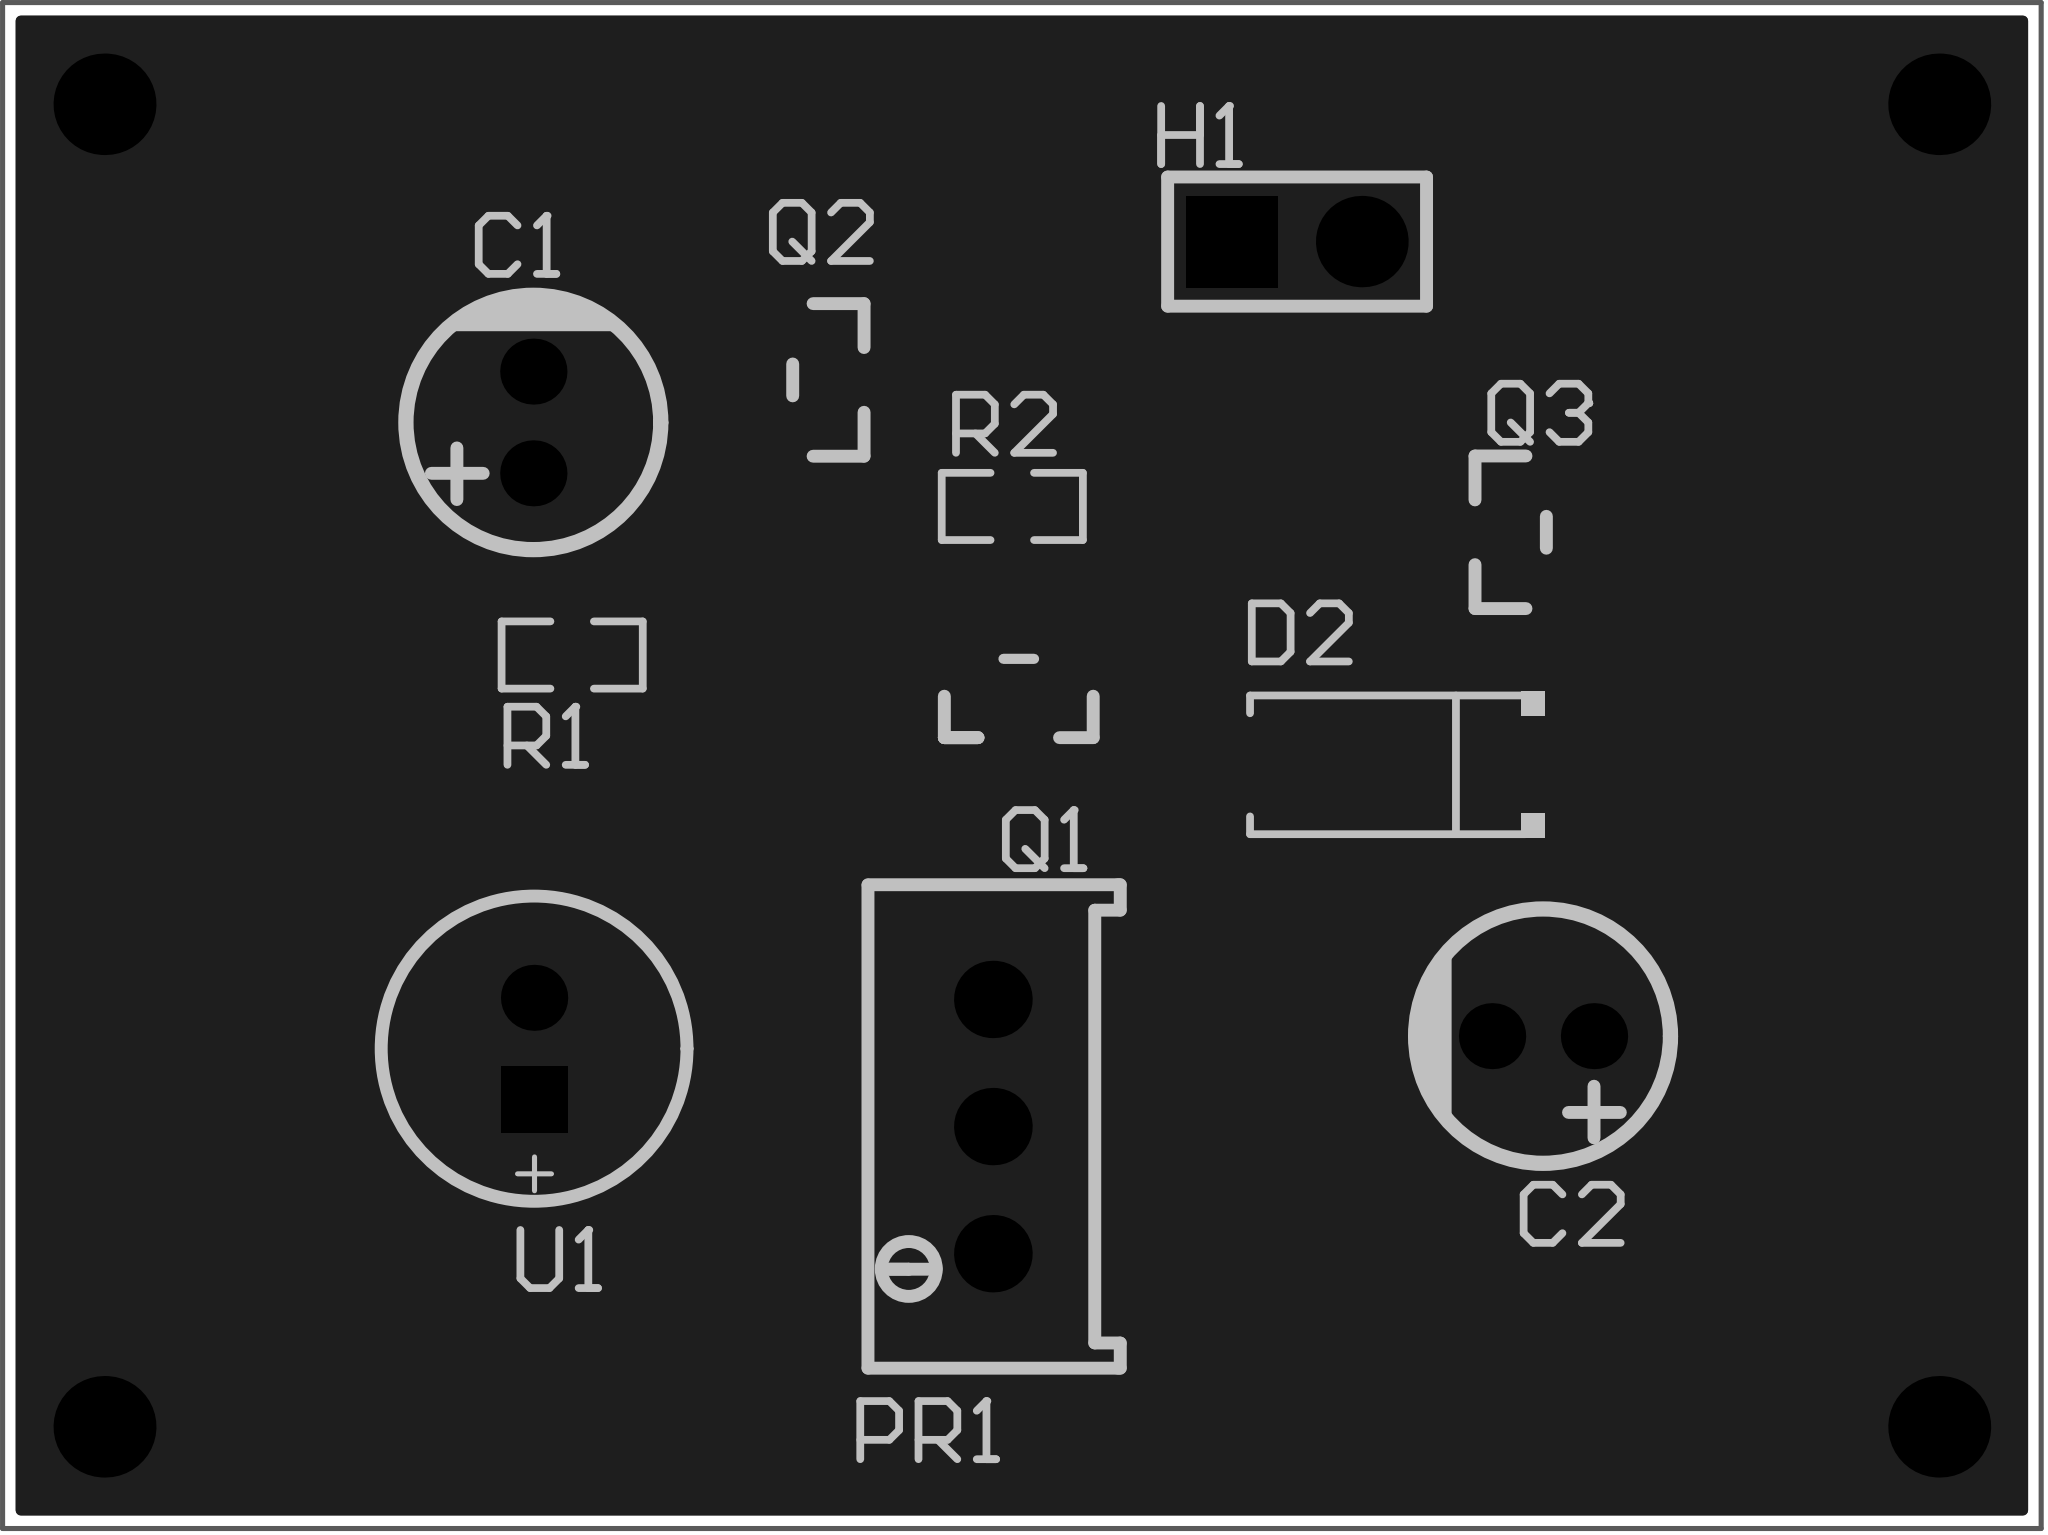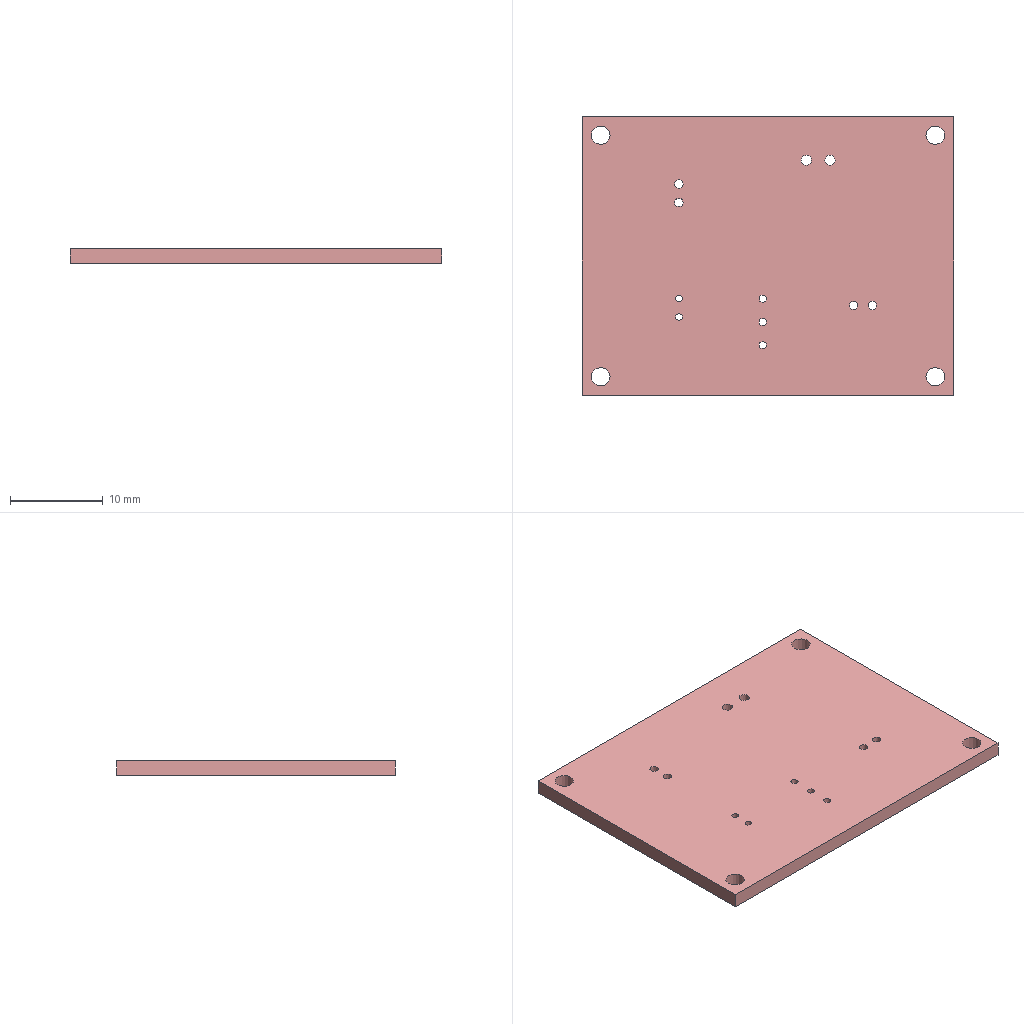Circuit board layout | Altium Designer | box 40 x 30 x 1.6 mm
Layer stack:
# Altium Designer layer stack of  (unit mm; dielectric type: 0 none, 1 core, 2 prepreg, 3 surface material)
index,name,kind,layer,copper_thickness_mm,dielectric_type,dielectric_thickness_mm,dielectric_material,dielectric_constant
0,Top Paste Mask Layer,other,,,,,,
1,Top Silkscreen Layer,other,,,,,,
2,Top Solder Mask Layer,dielectric,,,3,0.01,,3.3
3,Top Layer,copper,Top Layer,0.035,,,,
4,Dielectric1,dielectric,,,3,1.51,FR4,4.5
5,Bottom Layer,copper,Bottom Layer,0.035,,,,
6,Bottom Solder Mask Layer,dielectric,,,3,0.01,,3.3
7,Bottom Silkscreen Layer,other,,,,,,
8,Bottom Paste Mask Layer,other,,,,,,
# drill layer pairs: low layer,high layer
drill_pair,Top Layer,Bottom Layer
Part placement:
Designator,Comment,Layer,Footprint,Center-X(mm),Center-Y(mm),Rotation
C1,1uF,TopLayer,CAP-TH_BD5.0-P2.00-D0.8-FD-10UF50VC110GL,91.567,102.362,90
Q2,,TopLayer,S8050_SOT-23,97.356,103.198,180
C2,16v,TopLayer,CAP-TH_BD5.0-P2.00-D0.8-FD-10UF50VC110GL,111.379,90.297,180
H1,,TopLayer,HDR-TH_2P-P2.54-V-M-1,106.553,105.918,0
R2,10K,TopLayer,R0603,100.965,100.711,180
R1,10K,TopLayer,R0603,92.329,97.79,0
Q3,,TopLayer,S8050_SOT-23,110.744,100.203,0
Q1,,TopLayer,S8550P_SOT,101.092,96.816,90
U1,Current source,TopLayer,咪头,91.582,90.051,90
D2,,TopLayer,SMA_1N4007,108.331,95.631,180
PR1,10kΩ,TopLayer,R_3296,100.584,88.519,90
Pad and via stacks:
# Altium Designer via and pad stacks of  (unit mm). Each distinct definition once, with the count of objects using it.
# via: kind,start_layer,end_layer,hole_mm,diameter_mm,mode(0 simple;1 top-mid-bottom;2 full stack),diameter_per_layer,count,example_net
# pad: kind,layer,hole_mm,hole_type(0 round;1 square;2 slot),plating,top_size,top_shape(1 round;2 rect;3 octagon;9 rounded rect),mid_size,bottom_size,mode,footprint,size_per_layer,count,example
pad,Multi-Layer,0.9,0,plated,1.3x1.3,1,1.3x1.3,1.3x1.3,0,CAP-TH_BD5.0-P2.00-D0.8-FD-10UF50VC110GL,,4,C1.2
pad,Multi-Layer,2,0,plated,2x2,1,2x2,2x2,0,,,4,1
pad,Multi-Layer,1.1,0,plated,1.8x1.8,1,1.8x1.8,1.8x1.8,0,HDR-TH_2P-P2.54-V-M-1,,1,H1.2
pad,Multi-Layer,1.1,0,plated,1.8x1.8,2,1.8x1.8,1.8x1.8,0,HDR-TH_2P-P2.54-V-M-1,,1,H1.1
pad,Multi-Layer,0.7,0,plated,1.3x1.3,2,1.3x1.3,1.3x1.3,0,\u00DF\u00E4\u00CD\u00B7,,1,U1.1
pad,Multi-Layer,0.7,0,plated,1.3x1.3,1,1.3x1.3,1.3x1.3,0,\u00DF\u00E4\u00CD\u00B7,,1,U1.2
pad,Multi-Layer,0.762,0,plated,1.524x1.524,1,1.524x1.524,1.524x1.524,0,R_3296,,3,PR1.2
pad,Top Layer,0,0,plated,1x0.8,2,1x0.8,1x0.8,0,S8050_SOT-23,,6,Q2.2
pad,Top Layer,0,0,plated,0.8065x0.864,2,0.8065x0.864,0.8065x0.864,0,R0603,,4,R2.2
pad,Top Layer,0,0,plated,0.701x1.25,2,0.701x1.25,0.701x1.25,0,S8550P_SOT,,3,Q1.3
pad,Top Layer,0,0,plated,2.046x1.62,2,2.046x1.62,2.046x1.62,0,SMA_1N4007,,2,D2.2
Copper pours:
name,layer,net,type(0 solid;1 hatched;2 none)
Top Layer-GND,Top Layer,GND,0
Bottom Layer-GND,Bottom Layer,GND,0
Design rules, without the lines most boards share:
# Altium Designer design rules of  (exported by Altium Designer, unit mm)
# columns: name | kind | enabled | priority | scope1 | scope2 | descriptor | typed fields (field=value)
creepage | 65 | enabled | 1 | All | All | Creepage Distance Constraint =(0mil) (All),(All) |